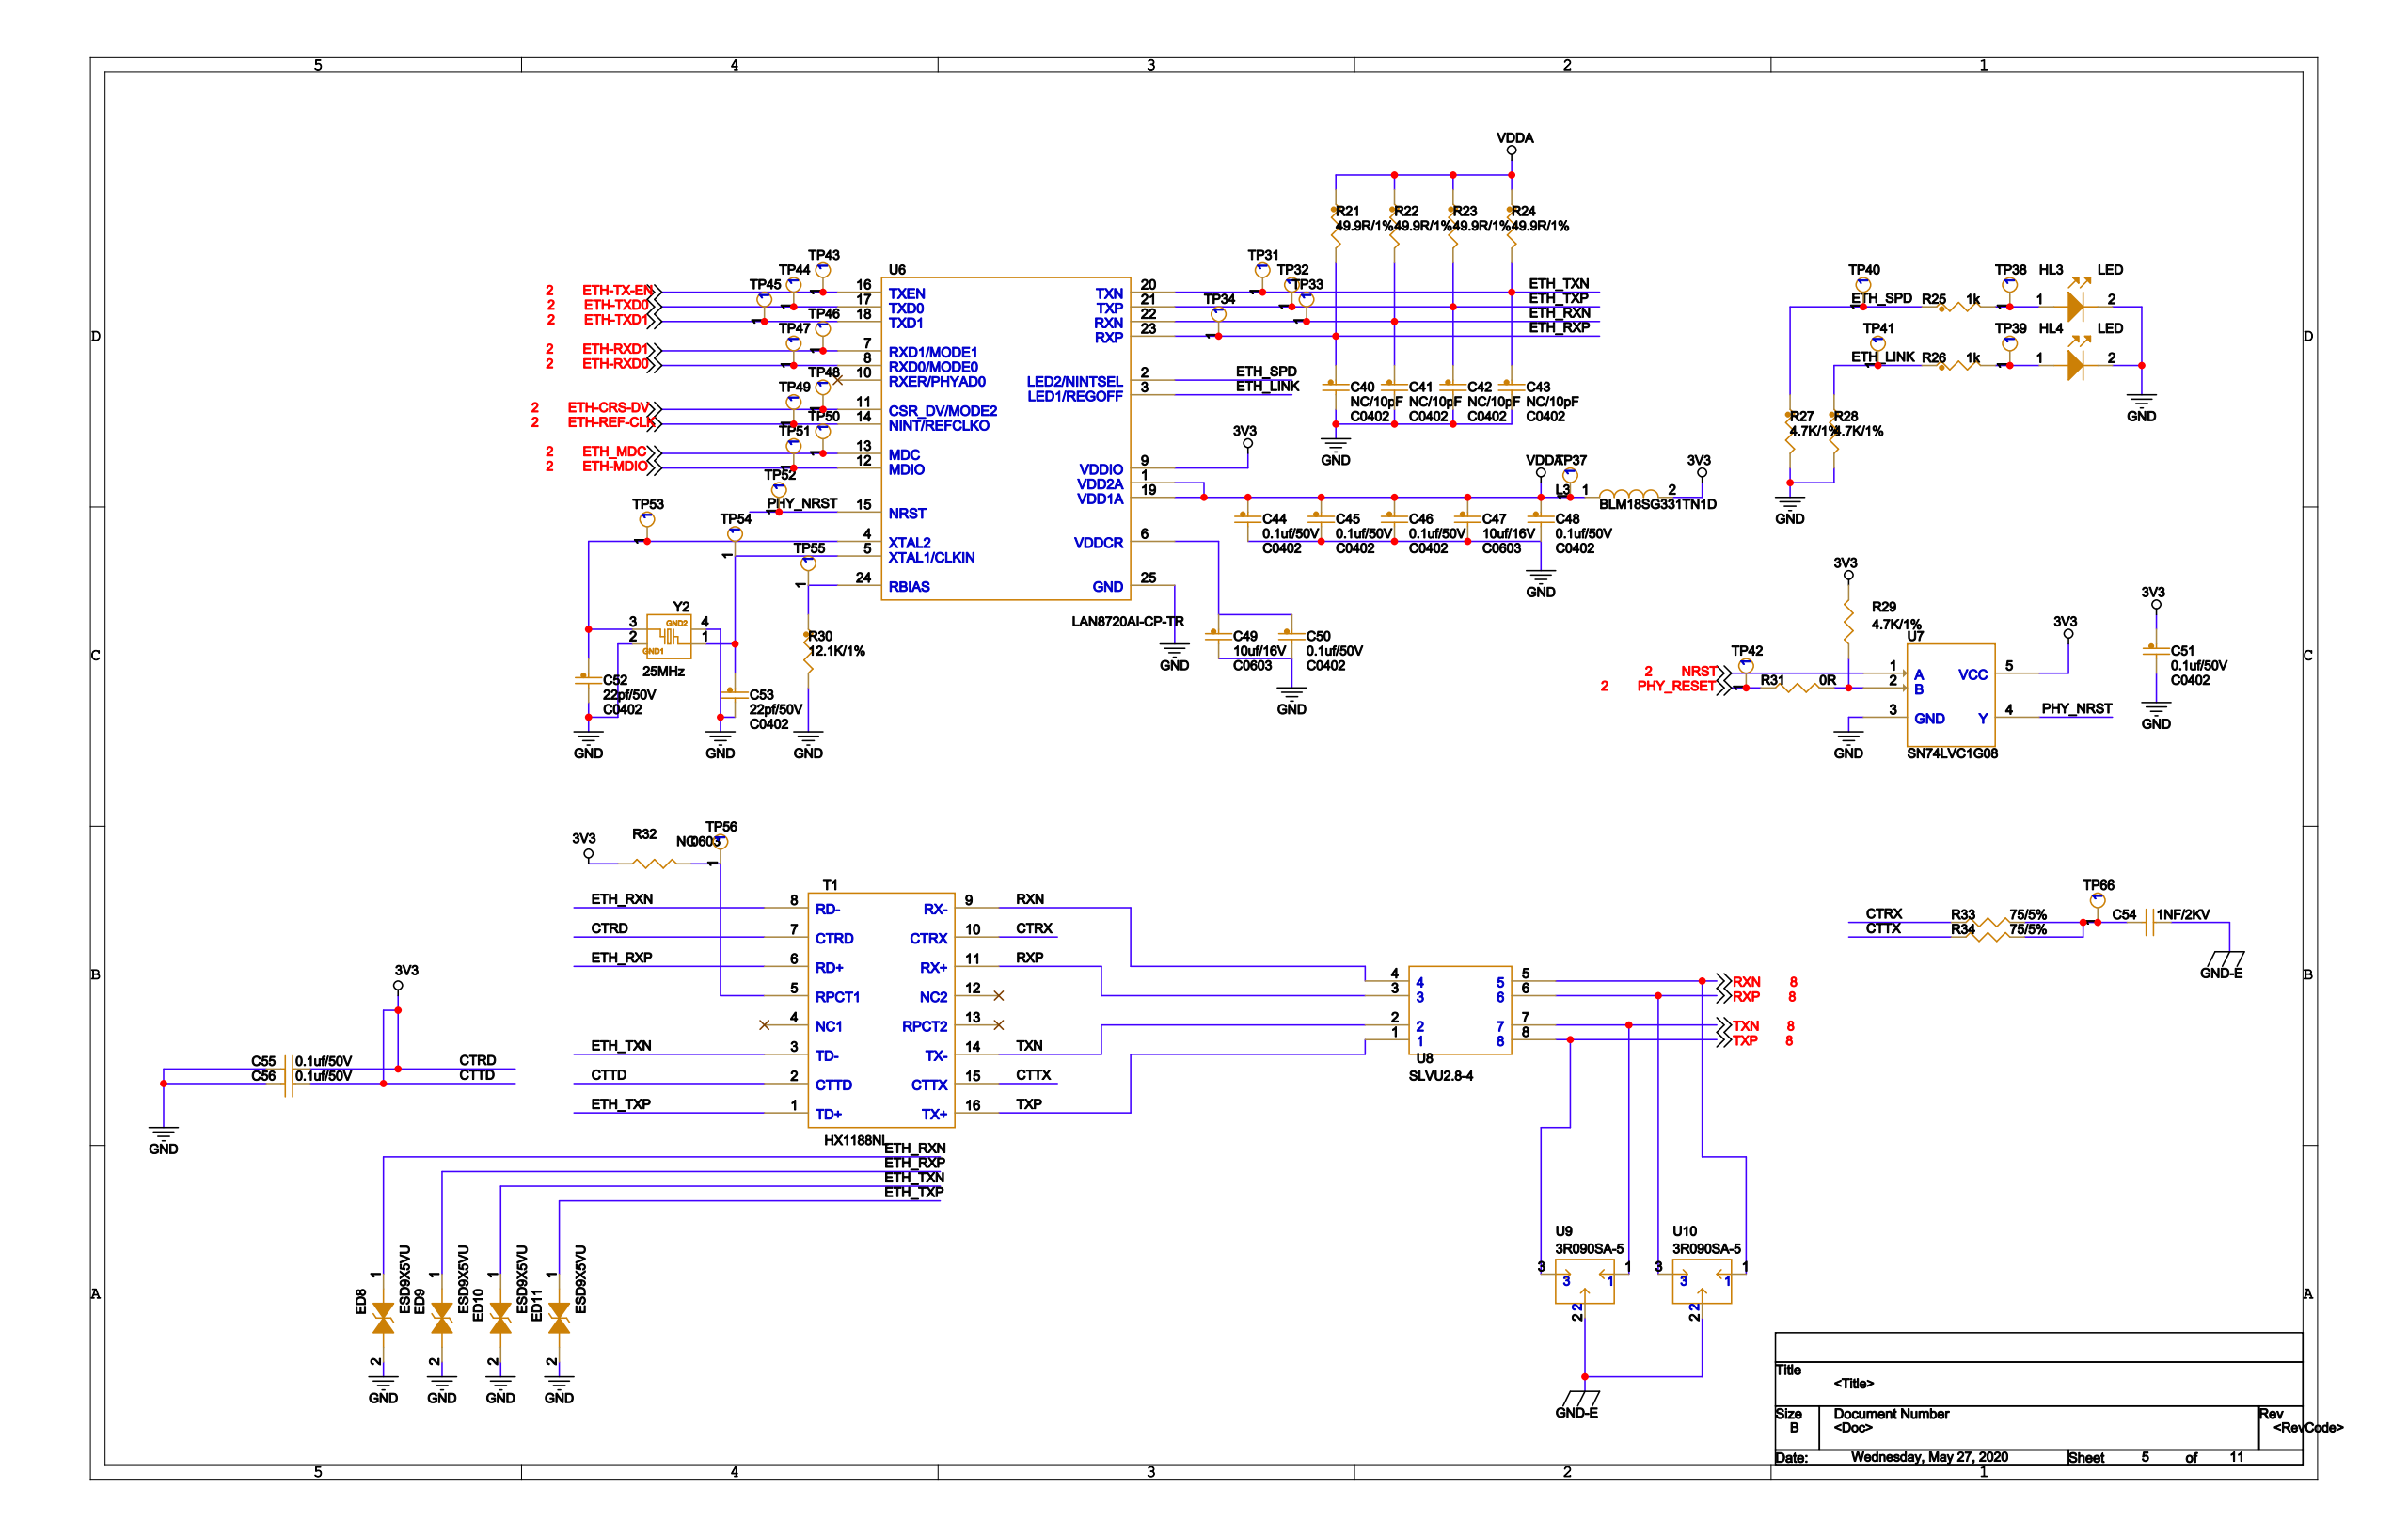Circuit board | Cadence Allegro | 521 parts | 239 nets | one sheet of the schematic
Parts on this sheet (reference | value | footprint):
C40 | NC/10pF | C0402
C41 | NC/10pF | C0402
C42 | NC/10pF | C0402
C43 | NC/10pF | C0402
C44 | 0.1uf/50V | C0402
C45 | 0.1uf/50V | C0402
C46 | 0.1uf/50V | C0402
C47 | 10uf/16V | C0603
C48 | 0.1uf/50V | C0402
C49 | 10uf/16V | C0603
C50 | 0.1uf/50V | C0402
C51 | 0.1uf/50V | C0402
C52 | 22pf/50V | C0402
C53 | 22pf/50V | C0402
C54 | 1NF/2KV | C1210
C55 | 0.1uf/50V | C0402
C56 | 0.1uf/50V | C0402
ED8 | ESD9X5VU | ESD5Z12T1
ED9 | ESD9X5VU | ESD5Z12T1
ED10 | ESD9X5VU | ESD5Z12T1
ED11 | ESD9X5VU | ESD5Z12T1
HL3 | LED | LED0603
HL4 | LED | LED0603
L3 | BLM18SG331TN1D | 0603
R21 | 49.9R/1% | 0603
R22 | 49.9R/1% | 0603
R23 | 49.9R/1% | 0603
R24 | 49.9R/1% | 0603
R25 | 1k | 0603
R26 | 1k | 0603
R27 | 4.7K/1% | 0402
R28 | 4.7K/1% | 0402
R29 | 4.7K/1% | 0402
R30 | 12.1K/1% | 0603
R31 | 0R | 0603
R32 | NC | 0603
R33 | 75/5% | 1206
R34 | 75/5% | 1206
T1 | HX1188NL | TRANS_H1102
TP31 | TESTPOINT | TESTPOINT-33MIL
TP32 | TESTPOINT | TESTPOINT-33MIL
TP33 | TESTPOINT | TESTPOINT-33MIL
TP34 | TESTPOINT | TESTPOINT-33MIL
TP37 | TESTPOINT | TESTPOINT-33MIL
TP38 | TESTPOINT | TESTPOINT-33MIL
TP39 | TESTPOINT | TESTPOINT-33MIL
TP40 | TESTPOINT | TESTPOINT-33MIL
TP41 | TESTPOINT | TESTPOINT-33MIL
TP42 | TESTPOINT | TESTPOINT-33MIL
TP43 | TESTPOINT | TESTPOINT-33MIL
TP44 | TESTPOINT | TESTPOINT-33MIL
TP45 | TESTPOINT | TESTPOINT-33MIL
TP46 | TESTPOINT | TESTPOINT-33MIL
TP47 | TESTPOINT | TESTPOINT-33MIL
TP48 | TESTPOINT | TESTPOINT-33MIL
TP49 | TESTPOINT | TESTPOINT-33MIL
TP50 | TESTPOINT | TESTPOINT-33MIL
TP51 | TESTPOINT | TESTPOINT-33MIL
TP52 | TESTPOINT | TESTPOINT-33MIL
TP53 | TESTPOINT | TESTPOINT-33MIL
TP54 | TESTPOINT | TESTPOINT-33MIL
TP55 | TESTPOINT | TESTPOINT-33MIL
TP56 | TESTPOINT | TESTPOINT-33MIL
TP66 | TESTPOINT | TESTPOINT-33MIL
U6 | LAN8720AI-CP-TR | QFN24
U7 | SN74LVC1G08 | SC70_5PIN
U8 | SLVU2.8-4 | SOP8
U9 | 3R090SA-5 | 3R090SA-5
U10 | 3R090SA-5 | 3R090SA-5
Y2 | 25MHz | OSC_SMD3L2X2L5
Nets of these parts (net: part-pin ...):
ETH_TXN: C43-1 ED10-1 R24-2 T1-3 TP31-1 U6-20
GND: C40-2 C41-2 C42-2 C43-2 C44-2 C45-2 C46-2 C47-2 C48-2 C49-2 C50-2 C51-2 C52-2 C53-2 C55-2 C56-2 ED8-2 ED9-2 ED10-2 ED11-2 HL3-2 HL4-2 R27-2 R28-2 R30-2 U7-3 Y2-2 Y2-4 U6-25
ETH_TXP: C42-1 ED11-1 R23-2 T1-1 TP32-1 U6-21
ETH_RXN: C41-1 ED8-1 R22-2 T1-8 TP33-1 U6-22
ETH_RXP: C40-1 ED9-1 R21-2 T1-6 TP34-1 U6-23
3V3: C51-1 C55-1 C56-1 L3-2 R29-2 R32-1 T1-2 T1-7 U7-5 U6-9
GND-E: C54-1 U9-2 U10-2
NRST: U7-1
VDDA: C44-1 C45-1 C46-1 C47-1 C48-1 L3-1 R21-1 R22-1 R23-1 R24-1 TP37-1 U6-1 U6-19
N7261762: HL3-1 R25-2 TP38-1
N7261772: HL4-1 R26-2 TP39-1
ETH_SPD: R25-1 R27-1 TP40-1 U6-2
ETH_LINK: R26-1 R28-1 TP41-1 U6-3
PHY_RESET: R31-1 TP42-1
ETH-TX-EN: TP43-1 U6-16
ETH-TXD0: TP44-1 U6-17
ETH-TXD1: TP45-1 U6-18
ETH-RXD1: TP46-1 U6-7
ETH-RXD0: TP47-1 U6-8
ETH-CRS-DV: TP48-1 U6-11
ETH-REF-CLK: TP49-1 U6-14
ETH_MDC: TP50-1 U6-13
ETH-MDIO: TP51-1 U6-12
PHY_NRST: TP52-1 U7-4 U6-15
N13416: C52-1 TP53-1 Y2-3 U6-4
N13448: C53-1 TP54-1 Y2-1 U6-5
N13556: R30-1 TP55-1 U6-24
N7186602: R32-2 T1-5 TP56-1
N7186980: C54-2 R33-2 R34-2 TP66-1
N7361898: R29-1 R31-2 U7-2
RXN: T1-9 U8-4 U8-5 U10-1
RXP: T1-11 U8-3 U8-6 U10-3
TXN: T1-14 U8-2 U8-7 U9-1
TXP: T1-16 U8-1 U8-8 U9-3
N15756: C49-1 C50-1 U6-6
CTRX: R33-1 T1-10
CTTX: R34-1 T1-15